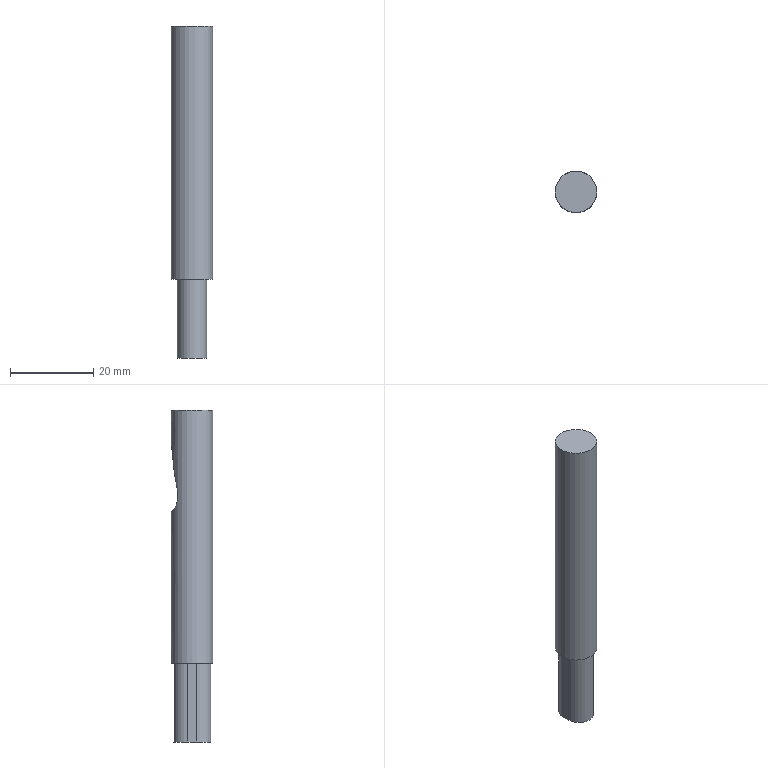Part | NX | features solid 2 | 1 solid | 11 faces | volume 5611 mm3 | plane 5 | cylinder 3 | sphere 2 | cone 1 | commonest cylinder face diameters 7 x2 10 x1